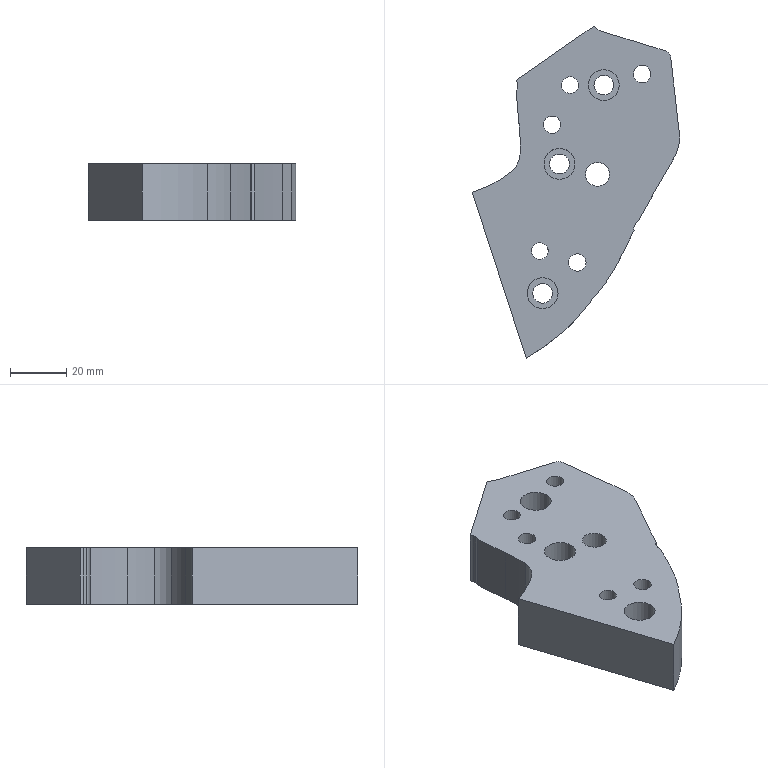Part | NX | features 23 2 | 1 solid | 44 faces | box 73.744 x 117.968 x 20 mm | volume 93989 mm3 | cylinder 30 | plane 14 | commonest cylinder face diameters 4.4 x4 6.2 x3 7 x3 11 x3 6.001 x2 5.6 x1
STEP:
#1=CARTESIAN_POINT('',(1173.772,235.011,-3.5));
#2=VERTEX_POINT('',#1);
#3=CARTESIAN_POINT('',(1169.522,235.011,-3.5));
#4=DIRECTION('',(0.,0.,-1.));
#5=DIRECTION('',(1.,0.,0.));
#6=AXIS2_PLACEMENT_3D('',#3,#4,#5);
#7=CIRCLE('',#6,4.25);
#8=EDGE_CURVE('',#2,#2,#7,.T.);
#9=ORIENTED_EDGE('',*,*,#8,.T.);
#10=EDGE_LOOP('',(#9));
#11=FACE_BOUND('',#10,.T.);
#12=CARTESIAN_POINT('',(1171.238,285.744,-3.5));
#13=VERTEX_POINT('',#12);
#14=CARTESIAN_POINT('',(1168.283,287.713,-3.5));
#15=VERTEX_POINT('',#14);
#16=CARTESIAN_POINT('',(1173.055,291.672,-3.5));
#17=DIRECTION('',(0.,0.,-1.));
#18=DIRECTION('',(-1.,0.,0.));
#19=AXIS2_PLACEMENT_3D('',#16,#17,#18);
#20=CIRCLE('',#19,6.2);
#21=EDGE_CURVE('',#13,#15,#20,.T.);
#22=ORIENTED_EDGE('',*,*,#21,.T.);
#23=CARTESIAN_POINT('',(1140.697,268.486,-3.5));
#24=VERTEX_POINT('',#23);
#25=CARTESIAN_POINT('',(1509.729,525.69,-3.5));
#26=DIRECTION('',(0.8204,0.5718,0.));
#27=VECTOR('',#26,1000.);
#28=LINE('',#25,#27);
#29=EDGE_CURVE('',#24,#15,#28,.T.);
#30=ORIENTED_EDGE('',*,*,#29,.F.);
#31=CARTESIAN_POINT('',(1141.067,267.339,-3.5));
#32=VERTEX_POINT('',#31);
#33=CARTESIAN_POINT('',(1138.868,267.263,-3.5));
#34=DIRECTION('',(0.,0.,-1.));
#35=DIRECTION('',(-1.,0.,0.));
#36=AXIS2_PLACEMENT_3D('',#33,#34,#35);
#37=CIRCLE('',#36,2.2);
#38=EDGE_CURVE('',#24,#32,#37,.T.);
#39=ORIENTED_EDGE('',*,*,#38,.T.);
#40=CARTESIAN_POINT('',(1141.104,266.344,-3.5));
#41=VERTEX_POINT('',#40);
#42=CARTESIAN_POINT('',(1326.856,273.811,-3.5));
#43=DIRECTION('',(0.,0.,1.));
#44=DIRECTION('',(-1.,0.,0.));
#45=AXIS2_PLACEMENT_3D('',#42,#43,#44);
#46=CIRCLE('',#45,185.901);
#47=EDGE_CURVE('',#32,#41,#46,.T.);
#48=ORIENTED_EDGE('',*,*,#47,.T.);
#49=CARTESIAN_POINT('',(1140.666,264.943,-3.5));
#50=VERTEX_POINT('',#49);
#51=CARTESIAN_POINT('',(1138.906,266.263,-3.5));
#52=DIRECTION('',(0.,0.,-1.));
#53=DIRECTION('',(-1.,0.,0.));
#54=AXIS2_PLACEMENT_3D('',#51,#52,#53);
#55=CIRCLE('',#54,2.2);
#56=EDGE_CURVE('',#41,#50,#55,.T.);
#57=ORIENTED_EDGE('',*,*,#56,.T.);
#58=CARTESIAN_POINT('',(1141.757,251.812,-3.5));
#59=VERTEX_POINT('',#58);
#60=CARTESIAN_POINT('',(1326.856,273.811,-3.5));
#61=DIRECTION('',(0.,0.,1.));
#62=DIRECTION('',(-1.,0.,0.));
#63=AXIS2_PLACEMENT_3D('',#60,#61,#62);
#64=CIRCLE('',#63,186.401);
#65=EDGE_CURVE('',#50,#59,#64,.T.);
#66=ORIENTED_EDGE('',*,*,#65,.T.);
#67=CARTESIAN_POINT('',(1141.998,242.228,-3.5));
#68=VERTEX_POINT('',#67);
#69=CARTESIAN_POINT('',(1057.602,244.9,-3.5));
#70=DIRECTION('',(0.,0.,-1.));
#71=DIRECTION('',(-1.,0.,0.));
#72=AXIS2_PLACEMENT_3D('',#69,#70,#71);
#73=CIRCLE('',#72,84.438);
#74=EDGE_CURVE('',#59,#68,#73,.T.);
#75=ORIENTED_EDGE('',*,*,#74,.T.);
#76=CARTESIAN_POINT('',(1139.107,236.023,-3.5));
#77=VERTEX_POINT('',#76);
#78=CARTESIAN_POINT('',(1132.519,242.868,-3.5));
#79=DIRECTION('',(0.,0.,-1.));
#80=DIRECTION('',(-1.,0.,0.));
#81=AXIS2_PLACEMENT_3D('',#78,#79,#80);
#82=CIRCLE('',#81,9.5);
#83=EDGE_CURVE('',#68,#77,#82,.T.);
#84=ORIENTED_EDGE('',*,*,#83,.T.);
#85=CARTESIAN_POINT('',(1131.001,231.048,-3.5));
#86=VERTEX_POINT('',#85);
#87=CARTESIAN_POINT('',(1115.023,266.175,-3.5));
#88=DIRECTION('',(0.,0.,-1.));
#89=DIRECTION('',(-1.,0.,0.));
#90=AXIS2_PLACEMENT_3D('',#87,#88,#89);
#91=CIRCLE('',#90,38.59);
#92=EDGE_CURVE('',#77,#86,#91,.T.);
#93=ORIENTED_EDGE('',*,*,#92,.T.);
#94=CARTESIAN_POINT('',(1126.024,229.046,-3.5));
#95=VERTEX_POINT('',#94);
#96=CARTESIAN_POINT('',(1126.024,229.046,-3.5));
#97=DIRECTION('',(-0.9278,-0.3732,0.));
#98=VECTOR('',#97,1000.);
#99=LINE('',#96,#98);
#100=EDGE_CURVE('',#86,#95,#99,.T.);
#101=ORIENTED_EDGE('',*,*,#100,.T.);
#102=CARTESIAN_POINT('',(1124.992,228.691,-3.5));
#103=VERTEX_POINT('',#102);
#104=CARTESIAN_POINT('',(597.176,1761.975,-3.5));
#105=DIRECTION('',(0.,0.,-1.));
#106=DIRECTION('',(-1.,0.,0.));
#107=AXIS2_PLACEMENT_3D('',#104,#105,#106);
#108=CIRCLE('',#107,1621.589);
#109=EDGE_CURVE('',#95,#103,#108,.T.);
#110=ORIENTED_EDGE('',*,*,#109,.T.);
#111=CARTESIAN_POINT('',(1144.11,169.745,-3.5));
#112=VERTEX_POINT('',#111);
#113=CARTESIAN_POINT('',(1110.681,272.818,-3.5));
#114=DIRECTION('',(0.3085,-0.9512,0.));
#115=VECTOR('',#114,1000.);
#116=LINE('',#113,#115);
#117=EDGE_CURVE('',#103,#112,#116,.T.);
#118=ORIENTED_EDGE('',*,*,#117,.T.);
#119=CARTESIAN_POINT('',(1167.22,190.006,-3.5));
#120=VERTEX_POINT('',#119);
#121=CARTESIAN_POINT('',(1111.807,229.9,-3.5));
#122=DIRECTION('',(0.,0.,1.));
#123=DIRECTION('',(-1.,0.,0.));
#124=AXIS2_PLACEMENT_3D('',#121,#122,#123);
#125=CIRCLE('',#124,68.28);
#126=EDGE_CURVE('',#112,#120,#125,.T.);
#127=ORIENTED_EDGE('',*,*,#126,.T.);
#128=CARTESIAN_POINT('',(1175.627,201.589,-3.5));
#129=VERTEX_POINT('',#128);
#130=CARTESIAN_POINT('',(1118.965,233.873,-3.5));
#131=DIRECTION('',(0.,0.,1.));
#132=DIRECTION('',(-1.,0.,0.));
#133=AXIS2_PLACEMENT_3D('',#130,#131,#132);
#134=CIRCLE('',#133,65.213);
#135=EDGE_CURVE('',#120,#129,#134,.T.);
#136=ORIENTED_EDGE('',*,*,#135,.T.);
#137=CARTESIAN_POINT('',(1182.483,215.038,-3.5));
#138=VERTEX_POINT('',#137);
#139=CARTESIAN_POINT('',(973.133,313.29,-3.5));
#140=DIRECTION('',(0.,0.,1.));
#141=DIRECTION('',(-1.,0.,0.));
#142=AXIS2_PLACEMENT_3D('',#139,#140,#141);
#143=CIRCLE('',#142,231.259);
#144=EDGE_CURVE('',#129,#138,#143,.T.);
#145=ORIENTED_EDGE('',*,*,#144,.T.);
#146=CARTESIAN_POINT('',(1182.612,216.501,-3.5));
#147=VERTEX_POINT('',#146);
#148=CARTESIAN_POINT('',(1184.614,215.586,-3.5));
#149=DIRECTION('',(0.,0.,-1.));
#150=DIRECTION('',(-1.,0.,0.));
#151=AXIS2_PLACEMENT_3D('',#148,#149,#150);
#152=CIRCLE('',#151,2.2);
#153=EDGE_CURVE('',#138,#147,#152,.T.);
#154=ORIENTED_EDGE('',*,*,#153,.T.);
#155=CARTESIAN_POINT('',(1183.03,217.409,-3.5));
#156=VERTEX_POINT('',#155);
#157=CARTESIAN_POINT('',(973.133,313.29,-3.5));
#158=DIRECTION('',(0.,0.,1.));
#159=DIRECTION('',(-1.,0.,0.));
#160=AXIS2_PLACEMENT_3D('',#157,#158,#159);
#161=CIRCLE('',#160,230.759);
#162=EDGE_CURVE('',#147,#156,#161,.T.);
#163=ORIENTED_EDGE('',*,*,#162,.T.);
#164=CARTESIAN_POINT('',(1184.097,218.487,-3.5));
#165=VERTEX_POINT('',#164);
#166=CARTESIAN_POINT('',(1185.031,216.495,-3.5));
#167=DIRECTION('',(0.,0.,-1.));
#168=DIRECTION('',(-1.,0.,0.));
#169=AXIS2_PLACEMENT_3D('',#166,#167,#168);
#170=CIRCLE('',#169,2.2);
#171=EDGE_CURVE('',#156,#165,#170,.T.);
#172=ORIENTED_EDGE('',*,*,#171,.T.);
#173=CARTESIAN_POINT('',(1193.968,236.067,-3.5));
#174=VERTEX_POINT('',#173);
#175=CARTESIAN_POINT('',(1664.113,-39.483,-3.5));
#176=DIRECTION('',(0.,0.,-1.));
#177=DIRECTION('',(-1.,0.,0.));
#178=AXIS2_PLACEMENT_3D('',#175,#176,#177);
#179=CIRCLE('',#178,544.944);
#180=EDGE_CURVE('',#165,#174,#179,.T.);
#181=ORIENTED_EDGE('',*,*,#180,.T.);
#182=CARTESIAN_POINT('',(1197.319,241.921,-3.5));
#183=VERTEX_POINT('',#182);
#184=CARTESIAN_POINT('',(1370.696,544.77,-3.5));
#185=DIRECTION('',(0.4968,0.8678,0.));
#186=VECTOR('',#185,1000.);
#187=LINE('',#184,#186);
#188=EDGE_CURVE('',#174,#183,#187,.T.);
#189=ORIENTED_EDGE('',*,*,#188,.T.);
#190=CARTESIAN_POINT('',(1198.437,250.945,-3.5));
#191=VERTEX_POINT('',#190);
#192=CARTESIAN_POINT('',(1184.704,248.065,-3.5));
#193=DIRECTION('',(0.,0.,1.));
#194=DIRECTION('',(-1.,0.,0.));
#195=AXIS2_PLACEMENT_3D('',#192,#193,#194);
#196=CIRCLE('',#195,14.032);
#197=EDGE_CURVE('',#183,#191,#196,.T.);
#198=ORIENTED_EDGE('',*,*,#197,.T.);
#199=CARTESIAN_POINT('',(1197.911,255.585,-3.5));
#200=VERTEX_POINT('',#199);
#201=CARTESIAN_POINT('',(1183.796,380.097,-3.5));
#202=DIRECTION('',(-0.1126,0.9936,0.));
#203=VECTOR('',#202,1000.);
#204=LINE('',#201,#203);
#205=EDGE_CURVE('',#191,#200,#204,.T.);
#206=ORIENTED_EDGE('',*,*,#205,.T.);
#207=CARTESIAN_POINT('',(1196.117,271.413,-3.5));
#208=VERTEX_POINT('',#207);
#209=CARTESIAN_POINT('',(1183.797,380.099,-3.5));
#210=DIRECTION('',(-0.1126,0.9936,0.));
#211=VECTOR('',#210,1000.);
#212=LINE('',#209,#211);
#213=EDGE_CURVE('',#200,#208,#212,.T.);
#214=ORIENTED_EDGE('',*,*,#213,.T.);
#215=CARTESIAN_POINT('',(1195.536,276.538,-3.5));
#216=VERTEX_POINT('',#215);
#217=CARTESIAN_POINT('',(1183.796,380.094,-3.5));
#218=DIRECTION('',(-0.1126,0.9936,0.));
#219=VECTOR('',#218,1000.);
#220=LINE('',#217,#219);
#221=EDGE_CURVE('',#208,#216,#220,.T.);
#222=ORIENTED_EDGE('',*,*,#221,.T.);
#223=CARTESIAN_POINT('',(1193.574,278.9,-3.5));
#224=VERTEX_POINT('',#223);
#225=CARTESIAN_POINT('',(1192.754,276.223,-3.5));
#226=DIRECTION('',(0.,0.,1.));
#227=DIRECTION('',(-1.,0.,0.));
#228=AXIS2_PLACEMENT_3D('',#225,#226,#227);
#229=CIRCLE('',#228,2.8);
#230=EDGE_CURVE('',#216,#224,#229,.T.);
#231=ORIENTED_EDGE('',*,*,#230,.T.);
#232=CARTESIAN_POINT('',(1182.916,282.165,-3.5));
#233=VERTEX_POINT('',#232);
#234=CARTESIAN_POINT('',(1505.832,183.228,-3.5));
#235=DIRECTION('',(-0.9561,0.2929,0.));
#236=VECTOR('',#235,1000.);
#237=LINE('',#234,#236);
#238=EDGE_CURVE('',#224,#233,#237,.T.);
#239=ORIENTED_EDGE('',*,*,#238,.T.);
#240=CARTESIAN_POINT('',(1505.815,183.216,-3.5));
#241=DIRECTION('',(-0.9561,0.293,0.));
#242=VECTOR('',#241,1000.);
#243=LINE('',#240,#242);
#244=EDGE_CURVE('',#233,#13,#243,.T.);
#245=ORIENTED_EDGE('',*,*,#244,.T.);
#246=EDGE_LOOP('',(#22,#30,#39,#48,#57,#66,#75,#84,#93,#101,#110,#118,#127,#136,#145,#154,#163,#172,#181,#189,#198,#206,#214,#222,#231,#239,#245));
#247=FACE_BOUND('',#246,.T.);
#248=CARTESIAN_POINT('',(1150.492,238.713,-3.5));
#249=VERTEX_POINT('',#248);
#250=CARTESIAN_POINT('',(1155.992,238.713,-3.5));
#251=DIRECTION('',(0.,0.,1.));
#252=DIRECTION('',(-1.,0.,0.));
#253=AXIS2_PLACEMENT_3D('',#250,#251,#252);
#254=CIRCLE('',#253,5.5);
#255=EDGE_CURVE('',#249,#249,#254,.T.);
#256=ORIENTED_EDGE('',*,*,#255,.F.);
#257=EDGE_LOOP('',(#256));
#258=FACE_BOUND('',#257,.T.);
#259=CARTESIAN_POINT('',(1144.492,192.745,-3.5));
#260=VERTEX_POINT('',#259);
#261=CARTESIAN_POINT('',(1149.992,192.745,-3.5));
#262=DIRECTION('',(0.,0.,1.));
#263=DIRECTION('',(-1.,0.,0.));
#264=AXIS2_PLACEMENT_3D('',#261,#262,#263);
#265=CIRCLE('',#264,5.5);
#266=EDGE_CURVE('',#260,#260,#265,.T.);
#267=ORIENTED_EDGE('',*,*,#266,.F.);
#268=EDGE_LOOP('',(#267));
#269=FACE_BOUND('',#268,.T.);
#270=CARTESIAN_POINT('',(1145.992,207.745,-3.5));
#271=VERTEX_POINT('',#270);
#272=CARTESIAN_POINT('',(1148.992,207.745,-3.5));
#273=DIRECTION('',(0.,0.,1.));
#274=DIRECTION('',(-1.,0.,0.));
#275=AXIS2_PLACEMENT_3D('',#272,#273,#274);
#276=CIRCLE('',#275,3.001);
#277=EDGE_CURVE('',#271,#271,#276,.T.);
#278=ORIENTED_EDGE('',*,*,#277,.F.);
#279=EDGE_LOOP('',(#278));
#280=FACE_BOUND('',#279,.T.);
#281=CARTESIAN_POINT('',(1166.236,266.713,-3.5));
#282=VERTEX_POINT('',#281);
#283=CARTESIAN_POINT('',(1171.736,266.713,-3.5));
#284=DIRECTION('',(0.,0.,1.));
#285=DIRECTION('',(-1.,0.,0.));
#286=AXIS2_PLACEMENT_3D('',#283,#284,#285);
#287=CIRCLE('',#286,5.5);
#288=EDGE_CURVE('',#282,#282,#287,.T.);
#289=ORIENTED_EDGE('',*,*,#288,.F.);
#290=EDGE_LOOP('',(#289));
#291=FACE_BOUND('',#290,.T.);
#292=CARTESIAN_POINT('',(1156.735,266.713,-3.5));
#293=VERTEX_POINT('',#292);
#294=CARTESIAN_POINT('',(1159.736,266.713,-3.5));
#295=DIRECTION('',(0.,0.,1.));
#296=DIRECTION('',(-1.,0.,0.));
#297=AXIS2_PLACEMENT_3D('',#294,#295,#296);
#298=CIRCLE('',#297,3.001);
#299=EDGE_CURVE('',#293,#293,#298,.T.);
#300=ORIENTED_EDGE('',*,*,#299,.F.);
#301=EDGE_LOOP('',(#300));
#302=FACE_BOUND('',#301,.T.);
#303=CARTESIAN_POINT('',(1159.26,203.637,-3.5));
#304=VERTEX_POINT('',#303);
#305=CARTESIAN_POINT('',(1162.36,203.637,-3.5));
#306=DIRECTION('',(0.,0.,1.));
#307=DIRECTION('',(-1.,0.,0.));
#308=AXIS2_PLACEMENT_3D('',#305,#306,#307);
#309=CIRCLE('',#308,3.1);
#310=EDGE_CURVE('',#304,#304,#309,.T.);
#311=ORIENTED_EDGE('',*,*,#310,.F.);
#312=EDGE_LOOP('',(#311));
#313=FACE_BOUND('',#312,.T.);
#314=CARTESIAN_POINT('',(1150.26,252.637,-3.5));
#315=VERTEX_POINT('',#314);
#316=CARTESIAN_POINT('',(1153.36,252.637,-3.5));
#317=DIRECTION('',(0.,0.,1.));
#318=DIRECTION('',(-1.,0.,0.));
#319=AXIS2_PLACEMENT_3D('',#316,#317,#318);
#320=CIRCLE('',#319,3.1);
#321=EDGE_CURVE('',#315,#315,#320,.T.);
#322=ORIENTED_EDGE('',*,*,#321,.F.);
#323=EDGE_LOOP('',(#322));
#324=FACE_BOUND('',#323,.T.);
#325=CARTESIAN_POINT('',(1182.26,270.637,-3.5));
#326=VERTEX_POINT('',#325);
#327=CARTESIAN_POINT('',(1185.36,270.637,-3.5));
#328=DIRECTION('',(0.,0.,1.));
#329=DIRECTION('',(-1.,0.,0.));
#330=AXIS2_PLACEMENT_3D('',#327,#328,#329);
#331=CIRCLE('',#330,3.1);
#332=EDGE_CURVE('',#326,#326,#331,.T.);
#333=ORIENTED_EDGE('',*,*,#332,.F.);
#334=EDGE_LOOP('',(#333));
#335=FACE_BOUND('',#334,.T.);
#336=CARTESIAN_POINT('',(1579.908,425.,-3.5));
#337=DIRECTION('',(0.,0.,-1.));
#338=DIRECTION('',(1.,0.,0.));
#339=AXIS2_PLACEMENT_3D('',#336,#337,#338);
#340=PLANE('',#339);
#341=ADVANCED_FACE('',(#11,#247,#258,#269,#280,#291,#302,#313,#324,#335),#340,.F.);
#342=CARTESIAN_POINT('',(1168.283,287.713,-23.5));
#343=VERTEX_POINT('',#342);
#344=CARTESIAN_POINT('',(1140.697,268.486,-23.5));
#345=VERTEX_POINT('',#344);
#346=CARTESIAN_POINT('',(996.344,167.876,-23.5));
#347=DIRECTION('',(-0.8204,-0.5718,0.));
#348=VECTOR('',#347,1000.);
#349=LINE('',#346,#348);
#350=EDGE_CURVE('',#343,#345,#349,.T.);
#351=ORIENTED_EDGE('',*,*,#350,.F.);
#352=CARTESIAN_POINT('',(1171.238,285.744,-23.5));
#353=VERTEX_POINT('',#352);
#354=CARTESIAN_POINT('',(1173.055,291.672,-23.5));
#355=DIRECTION('',(0.,0.,-1.));
#356=DIRECTION('',(-1.,0.,0.));
#357=AXIS2_PLACEMENT_3D('',#354,#355,#356);
#358=CIRCLE('',#357,6.2);
#359=EDGE_CURVE('',#353,#343,#358,.T.);
#360=ORIENTED_EDGE('',*,*,#359,.F.);
#361=CARTESIAN_POINT('',(1182.916,282.165,-23.5));
#362=VERTEX_POINT('',#361);
#363=CARTESIAN_POINT('',(1127.048,299.286,-23.5));
#364=DIRECTION('',(-0.9561,0.293,0.));
#365=VECTOR('',#364,1000.);
#366=LINE('',#363,#365);
#367=EDGE_CURVE('',#362,#353,#366,.T.);
#368=ORIENTED_EDGE('',*,*,#367,.F.);
#369=CARTESIAN_POINT('',(1193.574,278.9,-23.5));
#370=VERTEX_POINT('',#369);
#371=CARTESIAN_POINT('',(1127.048,299.282,-23.5));
#372=DIRECTION('',(0.9561,-0.2929,0.));
#373=VECTOR('',#372,1000.);
#374=LINE('',#371,#373);
#375=EDGE_CURVE('',#362,#370,#374,.T.);
#376=ORIENTED_EDGE('',*,*,#375,.T.);
#377=CARTESIAN_POINT('',(1195.536,276.538,-23.5));
#378=VERTEX_POINT('',#377);
#379=CARTESIAN_POINT('',(1192.754,276.223,-23.5));
#380=DIRECTION('',(0.,0.,1.));
#381=DIRECTION('',(-1.,0.,0.));
#382=AXIS2_PLACEMENT_3D('',#379,#380,#381);
#383=CIRCLE('',#382,2.8);
#384=EDGE_CURVE('',#378,#370,#383,.T.);
#385=ORIENTED_EDGE('',*,*,#384,.F.);
#386=CARTESIAN_POINT('',(1196.117,271.413,-23.5));
#387=VERTEX_POINT('',#386);
#388=CARTESIAN_POINT('',(1188.964,334.504,-23.5));
#389=DIRECTION('',(0.1126,-0.9936,0.));
#390=VECTOR('',#389,1000.);
#391=LINE('',#388,#390);
#392=EDGE_CURVE('',#378,#387,#391,.T.);
#393=ORIENTED_EDGE('',*,*,#392,.T.);
#394=CARTESIAN_POINT('',(1197.911,255.585,-23.5));
#395=VERTEX_POINT('',#394);
#396=CARTESIAN_POINT('',(1188.965,334.504,-23.5));
#397=DIRECTION('',(0.1126,-0.9936,0.));
#398=VECTOR('',#397,1000.);
#399=LINE('',#396,#398);
#400=EDGE_CURVE('',#387,#395,#399,.T.);
#401=ORIENTED_EDGE('',*,*,#400,.T.);
#402=CARTESIAN_POINT('',(1198.437,250.945,-23.5));
#403=VERTEX_POINT('',#402);
#404=CARTESIAN_POINT('',(1188.965,334.504,-23.5));
#405=DIRECTION('',(-0.1126,0.9936,0.));
#406=VECTOR('',#405,1000.);
#407=LINE('',#404,#406);
#408=EDGE_CURVE('',#403,#395,#407,.T.);
#409=ORIENTED_EDGE('',*,*,#408,.F.);
#410=CARTESIAN_POINT('',(1197.319,241.921,-23.5));
#411=VERTEX_POINT('',#410);
#412=CARTESIAN_POINT('',(1184.704,248.065,-23.5));
#413=DIRECTION('',(0.,0.,-1.));
#414=DIRECTION('',(-1.,0.,0.));
#415=AXIS2_PLACEMENT_3D('',#412,#413,#414);
#416=CIRCLE('',#415,14.032);
#417=EDGE_CURVE('',#403,#411,#416,.T.);
#418=ORIENTED_EDGE('',*,*,#417,.T.);
#419=CARTESIAN_POINT('',(1193.968,236.067,-23.5));
#420=VERTEX_POINT('',#419);
#421=CARTESIAN_POINT('',(1219.514,280.69,-23.5));
#422=DIRECTION('',(0.4968,0.8678,0.));
#423=VECTOR('',#422,1000.);
#424=LINE('',#421,#423);
#425=EDGE_CURVE('',#420,#411,#424,.T.);
#426=ORIENTED_EDGE('',*,*,#425,.F.);
#427=CARTESIAN_POINT('',(1184.097,218.487,-23.5));
#428=VERTEX_POINT('',#427);
#429=CARTESIAN_POINT('',(1664.113,-39.483,-23.5));
#430=DIRECTION('',(0.,0.,1.));
#431=DIRECTION('',(-1.,0.,0.));
#432=AXIS2_PLACEMENT_3D('',#429,#430,#431);
#433=CIRCLE('',#432,544.944);
#434=EDGE_CURVE('',#420,#428,#433,.T.);
#435=ORIENTED_EDGE('',*,*,#434,.T.);
#436=CARTESIAN_POINT('',(1183.03,217.409,-23.5));
#437=VERTEX_POINT('',#436);
#438=CARTESIAN_POINT('',(1185.031,216.495,-23.5));
#439=DIRECTION('',(0.,0.,-1.));
#440=DIRECTION('',(-1.,0.,0.));
#441=AXIS2_PLACEMENT_3D('',#438,#439,#440);
#442=CIRCLE('',#441,2.2);
#443=EDGE_CURVE('',#437,#428,#442,.T.);
#444=ORIENTED_EDGE('',*,*,#443,.F.);
#445=CARTESIAN_POINT('',(1182.612,216.501,-23.5));
#446=VERTEX_POINT('',#445);
#447=CARTESIAN_POINT('',(973.133,313.29,-23.5));
#448=DIRECTION('',(0.,0.,-1.));
#449=DIRECTION('',(-1.,0.,0.));
#450=AXIS2_PLACEMENT_3D('',#447,#448,#449);
#451=CIRCLE('',#450,230.759);
#452=EDGE_CURVE('',#437,#446,#451,.T.);
#453=ORIENTED_EDGE('',*,*,#452,.T.);
#454=CARTESIAN_POINT('',(1182.483,215.038,-23.5));
#455=VERTEX_POINT('',#454);
#456=CARTESIAN_POINT('',(1184.614,215.586,-23.5));
#457=DIRECTION('',(0.,0.,-1.));
#458=DIRECTION('',(-1.,0.,0.));
#459=AXIS2_PLACEMENT_3D('',#456,#457,#458);
#460=CIRCLE('',#459,2.2);
#461=EDGE_CURVE('',#455,#446,#460,.T.);
#462=ORIENTED_EDGE('',*,*,#461,.F.);
#463=CARTESIAN_POINT('',(1175.627,201.589,-23.5));
#464=VERTEX_POINT('',#463);
#465=CARTESIAN_POINT('',(973.133,313.29,-23.5));
#466=DIRECTION('',(0.,0.,1.));
#467=DIRECTION('',(-1.,0.,0.));
#468=AXIS2_PLACEMENT_3D('',#465,#466,#467);
#469=CIRCLE('',#468,231.259);
#470=EDGE_CURVE('',#464,#455,#469,.T.);
#471=ORIENTED_EDGE('',*,*,#470,.F.);
#472=CARTESIAN_POINT('',(1167.22,190.006,-23.5));
#473=VERTEX_POINT('',#472);
#474=CARTESIAN_POINT('',(1118.965,233.873,-23.5));
#475=DIRECTION('',(0.,0.,1.));
#476=DIRECTION('',(-1.,0.,0.));
#477=AXIS2_PLACEMENT_3D('',#474,#475,#476);
#478=CIRCLE('',#477,65.213);
#479=EDGE_CURVE('',#473,#464,#478,.T.);
#480=ORIENTED_EDGE('',*,*,#479,.F.);
#481=CARTESIAN_POINT('',(1144.11,169.745,-23.5));
#482=VERTEX_POINT('',#481);
#483=CARTESIAN_POINT('',(1111.807,229.9,-23.5));
#484=DIRECTION('',(0.,0.,-1.));
#485=DIRECTION('',(-1.,0.,0.));
#486=AXIS2_PLACEMENT_3D('',#483,#484,#485);
#487=CIRCLE('',#486,68.28);
#488=EDGE_CURVE('',#473,#482,#487,.T.);
#489=ORIENTED_EDGE('',*,*,#488,.T.);
#490=CARTESIAN_POINT('',(1124.992,228.691,-23.5));
#491=VERTEX_POINT('',#490);
#492=CARTESIAN_POINT('',(1143.323,172.172,-23.5));
#493=DIRECTION('',(-0.3085,0.9512,0.));
#494=VECTOR('',#493,1000.);
#495=LINE('',#492,#494);
#496=EDGE_CURVE('',#482,#491,#495,.T.);
#497=ORIENTED_EDGE('',*,*,#496,.T.);
#498=CARTESIAN_POINT('',(1126.024,229.046,-23.5));
#499=VERTEX_POINT('',#498);
#500=CARTESIAN_POINT('',(597.176,1761.975,-23.5));
#501=DIRECTION('',(0.,0.,-1.));
#502=DIRECTION('',(-1.,0.,0.));
#503=AXIS2_PLACEMENT_3D('',#500,#501,#502);
#504=CIRCLE('',#503,1621.589);
#505=EDGE_CURVE('',#499,#491,#504,.T.);
#506=ORIENTED_EDGE('',*,*,#505,.F.);
#507=CARTESIAN_POINT('',(1131.001,231.048,-23.5));
#508=VERTEX_POINT('',#507);
#509=CARTESIAN_POINT('',(1169.044,246.35,-23.5));
#510=DIRECTION('',(-0.9278,-0.3732,0.));
#511=VECTOR('',#510,1000.);
#512=LINE('',#509,#511);
#513=EDGE_CURVE('',#508,#499,#512,.T.);
#514=ORIENTED_EDGE('',*,*,#513,.F.);
#515=CARTESIAN_POINT('',(1139.107,236.023,-23.5));
#516=VERTEX_POINT('',#515);
#517=CARTESIAN_POINT('',(1115.023,266.175,-23.5));
#518=DIRECTION('',(0.,0.,1.));
#519=DIRECTION('',(-1.,0.,0.));
#520=AXIS2_PLACEMENT_3D('',#517,#518,#519);
#521=CIRCLE('',#520,38.59);
#522=EDGE_CURVE('',#508,#516,#521,.T.);
#523=ORIENTED_EDGE('',*,*,#522,.T.);
#524=CARTESIAN_POINT('',(1141.998,242.228,-23.5));
#525=VERTEX_POINT('',#524);
#526=CARTESIAN_POINT('',(1132.519,242.868,-23.5));
#527=DIRECTION('',(0.,0.,-1.));
#528=DIRECTION('',(-1.,0.,0.));
#529=AXIS2_PLACEMENT_3D('',#526,#527,#528);
#530=CIRCLE('',#529,9.5);
#531=EDGE_CURVE('',#525,#516,#530,.T.);
#532=ORIENTED_EDGE('',*,*,#531,.F.);
#533=CARTESIAN_POINT('',(1141.757,251.812,-23.5));
#534=VERTEX_POINT('',#533);
#535=CARTESIAN_POINT('',(1057.602,244.9,-23.5));
#536=DIRECTION('',(0.,0.,1.));
#537=DIRECTION('',(-1.,0.,0.));
#538=AXIS2_PLACEMENT_3D('',#535,#536,#537);
#539=CIRCLE('',#538,84.438);
#540=EDGE_CURVE('',#525,#534,#539,.T.);
#541=ORIENTED_EDGE('',*,*,#540,.T.);
#542=CARTESIAN_POINT('',(1140.666,264.943,-23.5));
#543=VERTEX_POINT('',#542);
#544=CARTESIAN_POINT('',(1326.856,273.811,-23.5));
#545=DIRECTION('',(0.,0.,-1.));
#546=DIRECTION('',(-1.,0.,0.));
#547=AXIS2_PLACEMENT_3D('',#544,#545,#546);
#548=CIRCLE('',#547,186.401);
#549=EDGE_CURVE('',#534,#543,#548,.T.);
#550=ORIENTED_EDGE('',*,*,#549,.T.);
#551=CARTESIAN_POINT('',(1141.104,266.344,-23.5));
#552=VERTEX_POINT('',#551);
#553=CARTESIAN_POINT('',(1138.906,266.263,-23.5));
#554=DIRECTION('',(0.,0.,-1.));
#555=DIRECTION('',(-1.,0.,0.));
#556=AXIS2_PLACEMENT_3D('',#553,#554,#555);
#557=CIRCLE('',#556,2.2);
#558=EDGE_CURVE('',#552,#543,#557,.T.);
#559=ORIENTED_EDGE('',*,*,#558,.F.);
#560=CARTESIAN_POINT('',(1141.067,267.339,-23.5));
#561=VERTEX_POINT('',#560);
#562=CARTESIAN_POINT('',(1326.856,273.811,-23.5));
#563=DIRECTION('',(0.,0.,-1.));
#564=DIRECTION('',(-1.,0.,0.));
#565=AXIS2_PLACEMENT_3D('',#562,#563,#564);
#566=CIRCLE('',#565,185.901);
#567=EDGE_CURVE('',#552,#561,#566,.T.);
#568=ORIENTED_EDGE('',*,*,#567,.T.);
#569=CARTESIAN_POINT('',(1138.868,267.263,-23.5));
#570=DIRECTION('',(0.,0.,-1.));
#571=DIRECTION('',(-1.,0.,0.));
#572=AXIS2_PLACEMENT_3D('',#569,#570,#571);
#573=CIRCLE('',#572,2.2);
#574=EDGE_CURVE('',#345,#561,#573,.T.);
#575=ORIENTED_EDGE('',*,*,#574,.F.);
#576=EDGE_LOOP('',(#351,#360,#368,#376,#385,#393,#401,#409,#418,#426,#435,#444,#453,#462,#471,#480,#489,#497,#506,#514,#523,#532,#541,#550,#559,#568,#575));
#577=FACE_BOUND('',#576,.T.);
#578=CARTESIAN_POINT('',(1152.492,238.713,-23.5));
#579=VERTEX_POINT('',#578);
#580=CARTESIAN_POINT('',(1155.992,238.713,-23.5));
#581=DIRECTION('',(0.,0.,1.));
#582=DIRECTION('',(-1.,0.,0.));
#583=AXIS2_PLACEMENT_3D('',#580,#581,#582);
#584=CIRCLE('',#583,3.5);
#585=EDGE_CURVE('',#579,#579,#584,.T.);
#586=ORIENTED_EDGE('',*,*,#585,.T.);
#587=EDGE_LOOP('',(#586));
#588=FACE_BOUND('',#587,.T.);
#589=CARTESIAN_POINT('',(1146.492,192.745,-23.5));
#590=VERTEX_POINT('',#589);
#591=CARTESIAN_POINT('',(1149.992,192.745,-23.5));
#592=DIRECTION('',(0.,0.,1.));
#593=DIRECTION('',(-1.,0.,0.));
#594=AXIS2_PLACEMENT_3D('',#591,#592,#593);
#595=CIRCLE('',#594,3.5);
#596=EDGE_CURVE('',#590,#590,#595,.T.);
#597=ORIENTED_EDGE('',*,*,#596,.T.);
#598=EDGE_LOOP('',(#597));
#599=FACE_BOUND('',#598,.T.);
#600=CARTESIAN_POINT('',(1145.992,207.745,-23.5));
#601=VERTEX_POINT('',#600);
#602=CARTESIAN_POINT('',(1148.992,207.745,-23.5));
#603=DIRECTION('',(0.,0.,1.));
#604=DIRECTION('',(-1.,0.,0.));
#605=AXIS2_PLACEMENT_3D('',#602,#603,#604);
#606=CIRCLE('',#605,3.001);
#607=EDGE_CURVE('',#601,#601,#606,.T.);
#608=ORIENTED_EDGE('',*,*,#607,.T.);
#609=EDGE_LOOP('',(#608));
#610=FACE_BOUND('',#609,.T.);
#611=CARTESIAN_POINT('',(1168.236,266.713,-23.5));
#612=VERTEX_POINT('',#611);
#613=CARTESIAN_POINT('',(1171.736,266.713,-23.5));
#614=DIRECTION('',(0.,0.,1.));
#615=DIRECTION('',(-1.,0.,0.));
#616=AXIS2_PLACEMENT_3D('',#613,#614,#615);
#617=CIRCLE('',#616,3.5);
#618=EDGE_CURVE('',#612,#612,#617,.T.);
#619=ORIENTED_EDGE('',*,*,#618,.T.);
#620=EDGE_LOOP('',(#619));
#621=FACE_BOUND('',#620,.T.);
#622=CARTESIAN_POINT('',(1156.735,266.713,-23.5));
#623=VERTEX_POINT('',#622);
#624=CARTESIAN_POINT('',(1159.736,266.713,-23.5));
#625=DIRECTION('',(0.,0.,1.));
#626=DIRECTION('',(-1.,0.,0.));
#627=AXIS2_PLACEMENT_3D('',#624,#625,#626);
#628=CIRCLE('',#627,3.001);
#629=EDGE_CURVE('',#623,#623,#628,.T.);
#630=ORIENTED_EDGE('',*,*,#629,.T.);
#631=EDGE_LOOP('',(#630));
#632=FACE_BOUND('',#631,.T.);
#633=CARTESIAN_POINT('',(1159.26,203.637,-23.5));
#634=VERTEX_POINT('',#633);
#635=CARTESIAN_POINT('',(1162.36,203.637,-23.5));
#636=DIRECTION('',(0.,0.,1.));
#637=DIRECTION('',(-1.,0.,0.));
#638=AXIS2_PLACEMENT_3D('',#635,#636,#637);
#639=CIRCLE('',#638,3.1);
#640=EDGE_CURVE('',#634,#634,#639,.T.);
#641=ORIENTED_EDGE('',*,*,#640,.T.);
#642=EDGE_LOOP('',(#641));
#643=FACE_BOUND('',#642,.T.);
#644=CARTESIAN_POINT('',(1150.26,252.637,-23.5));
#645=VERTEX_POINT('',#644);
#646=CARTESIAN_POINT('',(1153.36,252.637,-23.5));
#647=DIRECTION('',(0.,0.,1.));
#648=DIRECTION('',(-1.,0.,0.));
#649=AXIS2_PLACEMENT_3D('',#646,#647,#648);
#650=CIRCLE('',#649,3.1);
#651=EDGE_CURVE('',#645,#645,#650,.T.);
#652=ORIENTED_EDGE('',*,*,#651,.T.);
#653=EDGE_LOOP('',(#652));
#654=FACE_BOUND('',#653,.T.);
#655=CARTESIAN_POINT('',(1182.26,270.637,-23.5));
#656=VERTEX_POINT('',#655);
#657=CARTESIAN_POINT('',(1185.36,270.637,-23.5));
#658=DIRECTION('',(0.,0.,1.));
#659=DIRECTION('',(-1.,0.,0.));
#660=AXIS2_PLACEMENT_3D('',#657,#658,#659);
#661=CIRCLE('',#660,3.1);
#662=EDGE_CURVE('',#656,#656,#661,.T.);
#663=ORIENTED_EDGE('',*,*,#662,.T.);
#664=EDGE_LOOP('',(#663));
#665=FACE_BOUND('',#664,.T.);
#666=CARTESIAN_POINT('',(1165.272,235.011,-23.5));
#667=VERTEX_POINT('',#666);
#668=CARTESIAN_POINT('',(1169.522,235.011,-23.5));
#669=DIRECTION('',(0.,0.,1.));
#670=DIRECTION('',(-1.,0.,0.));
#671=AXIS2_PLACEMENT_3D('',#668,#669,#670);
#672=CIRCLE('',#671,4.25);
#673=EDGE_CURVE('',#667,#667,#672,.T.);
#674=ORIENTED_EDGE('',*,*,#673,.T.);
#675=EDGE_LOOP('',(#674));
#676=FACE_BOUND('',#675,.T.);
#677=CARTESIAN_POINT('',(1021.,132.5,-23.5));
#678=DIRECTION('',(0.,0.,-1.));
#679=DIRECTION('',(1.,0.,0.));
#680=AXIS2_PLACEMENT_3D('',#677,#678,#679);
#681=PLANE('',#680);
#682=ADVANCED_FACE('',(#577,#588,#599,#610,#621,#632,#643,#654,#665,#676),#681,.T.);
#683=ORIENTED_EDGE('',*,*,#479,.T.);
#684=CARTESIAN_POINT('',(1175.627,201.589,-43.));
#685=DIRECTION('',(0.,0.,-1.));
#686=VECTOR('',#685,1000.);
#687=LINE('',#684,#686);
#688=EDGE_CURVE('',#129,#464,#687,.T.);
#689=ORIENTED_EDGE('',*,*,#688,.F.);
#690=ORIENTED_EDGE('',*,*,#135,.F.);
#691=CARTESIAN_POINT('',(1167.22,190.006,-43.));
#692=DIRECTION('',(0.,0.,-1.));
#693=VECTOR('',#692,1000.);
#694=LINE('',#691,#693);
#695=EDGE_CURVE('',#120,#473,#694,.T.);
#696=ORIENTED_EDGE('',*,*,#695,.T.);
#697=EDGE_LOOP('',(#683,#689,#690,#696));
#698=FACE_BOUND('',#697,.T.);
#699=CARTESIAN_POINT('',(1118.965,233.873,-43.));
#700=DIRECTION('',(0.,0.,1.));
#701=DIRECTION('',(-1.,0.,0.));
#702=AXIS2_PLACEMENT_3D('',#699,#700,#701);
#703=CYLINDRICAL_SURFACE('',#702,65.213);
#704=ADVANCED_FACE('',(#698),#703,.T.);
#705=ORIENTED_EDGE('',*,*,#470,.T.);
#706=CARTESIAN_POINT('',(1182.483,215.038,-43.));
#707=DIRECTION('',(0.,0.,-1.));
#708=VECTOR('',#707,1000.);
#709=LINE('',#706,#708);
#710=EDGE_CURVE('',#138,#455,#709,.T.);
#711=ORIENTED_EDGE('',*,*,#710,.F.);
#712=ORIENTED_EDGE('',*,*,#144,.F.);
#713=ORIENTED_EDGE('',*,*,#688,.T.);
#714=EDGE_LOOP('',(#705,#711,#712,#713));
#715=FACE_BOUND('',#714,.T.);
#716=CARTESIAN_POINT('',(973.133,313.29,-43.));
#717=DIRECTION('',(0.,0.,1.));
#718=DIRECTION('',(-1.,0.,0.));
#719=AXIS2_PLACEMENT_3D('',#716,#717,#718);
#720=CYLINDRICAL_SURFACE('',#719,231.259);
#721=ADVANCED_FACE('',(#715),#720,.T.);
#722=ORIENTED_EDGE('',*,*,#461,.T.);
#723=CARTESIAN_POINT('',(1182.612,216.501,-23.5));
#724=CARTESIAN_POINT('',(1182.612,216.501,-16.833));
#725=CARTESIAN_POINT('',(1182.612,216.501,-10.167));
#726=CARTESIAN_POINT('',(1182.612,216.501,-3.5));
#727=B_SPLINE_CURVE_WITH_KNOTS('',3,(#723,#724,#725,#726),.UNSPECIFIED.,.F.,.F.,(4,4),(0.,1.),.UNSPECIFIED.);
#728=EDGE_CURVE('',#147,#446,#727,.F.);
#729=ORIENTED_EDGE('',*,*,#728,.F.);
#730=ORIENTED_EDGE('',*,*,#153,.F.);
#731=ORIENTED_EDGE('',*,*,#710,.T.);
#732=EDGE_LOOP('',(#722,#729,#730,#731));
#733=FACE_BOUND('',#732,.T.);
#734=CARTESIAN_POINT('',(1184.614,215.586,-43.));
#735=DIRECTION('',(0.,0.,1.));
#736=DIRECTION('',(-1.,0.,0.));
#737=AXIS2_PLACEMENT_3D('',#734,#735,#736);
#738=CYLINDRICAL_SURFACE('',#737,2.2);
#739=ADVANCED_FACE('',(#733),#738,.F.);
#740=ORIENTED_EDGE('',*,*,#452,.F.);
#741=CARTESIAN_POINT('',(1183.03,217.409,-43.));
#742=DIRECTION('',(0.,0.,-1.));
#743=VECTOR('',#742,1000.);
#744=LINE('',#741,#743);
#745=EDGE_CURVE('',#156,#437,#744,.T.);
#746=ORIENTED_EDGE('',*,*,#745,.F.);
#747=ORIENTED_EDGE('',*,*,#162,.F.);
#748=ORIENTED_EDGE('',*,*,#728,.T.);
#749=EDGE_LOOP('',(#740,#746,#747,#748));
#750=FACE_BOUND('',#749,.T.);
#751=CARTESIAN_POINT('',(973.133,313.29,-43.));
#752=DIRECTION('',(0.,0.,1.));
#753=DIRECTION('',(-1.,0.,0.));
#754=AXIS2_PLACEMENT_3D('',#751,#752,#753);
#755=CYLINDRICAL_SURFACE('',#754,230.759);
#756=ADVANCED_FACE('',(#750),#755,.T.);
#757=ORIENTED_EDGE('',*,*,#443,.T.);
#758=CARTESIAN_POINT('',(1184.097,218.487,-43.));
#759=DIRECTION('',(0.,0.,-1.));
#760=VECTOR('',#759,1000.);
#761=LINE('',#758,#760);
#762=EDGE_CURVE('',#165,#428,#761,.T.);
#763=ORIENTED_EDGE('',*,*,#762,.F.);
#764=ORIENTED_EDGE('',*,*,#171,.F.);
#765=ORIENTED_EDGE('',*,*,#745,.T.);
#766=EDGE_LOOP('',(#757,#763,#764,#765));
#767=FACE_BOUND('',#766,.T.);
#768=CARTESIAN_POINT('',(1185.031,216.495,-43.));
#769=DIRECTION('',(0.,0.,1.));
#770=DIRECTION('',(-1.,0.,0.));
#771=AXIS2_PLACEMENT_3D('',#768,#769,#770);
#772=CYLINDRICAL_SURFACE('',#771,2.2);
#773=ADVANCED_FACE('',(#767),#772,.F.);
#774=ORIENTED_EDGE('',*,*,#434,.F.);
#775=CARTESIAN_POINT('',(1193.968,236.067,-43.));
#776=DIRECTION('',(0.,0.,-1.));
#777=VECTOR('',#776,1000.);
#778=LINE('',#775,#777);
#779=EDGE_CURVE('',#174,#420,#778,.T.);
#780=ORIENTED_EDGE('',*,*,#779,.F.);
#781=ORIENTED_EDGE('',*,*,#180,.F.);
#782=ORIENTED_EDGE('',*,*,#762,.T.);
#783=EDGE_LOOP('',(#774,#780,#781,#782));
#784=FACE_BOUND('',#783,.T.);
#785=CARTESIAN_POINT('',(1664.113,-39.483,-43.));
#786=DIRECTION('',(0.,0.,1.));
#787=DIRECTION('',(-1.,0.,0.));
#788=AXIS2_PLACEMENT_3D('',#785,#786,#787);
#789=CYLINDRICAL_SURFACE('',#788,544.944);
#790=ADVANCED_FACE('',(#784),#789,.F.);
#791=ORIENTED_EDGE('',*,*,#425,.T.);
#792=CARTESIAN_POINT('',(1197.319,241.921,-13.5));
#793=DIRECTION('',(0.,0.,-1.));
#794=VECTOR('',#793,1000.);
#795=LINE('',#792,#794);
#796=EDGE_CURVE('',#183,#411,#795,.T.);
#797=ORIENTED_EDGE('',*,*,#796,.F.);
#798=ORIENTED_EDGE('',*,*,#188,.F.);
#799=ORIENTED_EDGE('',*,*,#779,.T.);
#800=EDGE_LOOP('',(#791,#797,#798,#799));
#801=FACE_BOUND('',#800,.T.);
#802=CARTESIAN_POINT('',(1193.968,236.067,-43.));
#803=DIRECTION('',(0.8678,-0.4968,0.));
#804=DIRECTION('',(-0.4968,-0.8678,0.));
#805=AXIS2_PLACEMENT_3D('',#802,#803,#804);
#806=PLANE('',#805);
#807=ADVANCED_FACE('',(#801),#806,.T.);
#808=ORIENTED_EDGE('',*,*,#417,.F.);
#809=CARTESIAN_POINT('',(1198.437,250.945,-3.5));
#810=DIRECTION('',(0.,0.,1.));
#811=VECTOR('',#810,1000.);
#812=LINE('',#809,#811);
#813=EDGE_CURVE('',#191,#403,#812,.F.);
#814=ORIENTED_EDGE('',*,*,#813,.F.);
#815=ORIENTED_EDGE('',*,*,#197,.F.);
#816=ORIENTED_EDGE('',*,*,#796,.T.);
#817=EDGE_LOOP('',(#808,#814,#815,#816));
#818=FACE_BOUND('',#817,.T.);
#819=CARTESIAN_POINT('',(1184.704,248.065,-43.));
#820=DIRECTION('',(0.,0.,1.));
#821=DIRECTION('',(-1.,0.,0.));
#822=AXIS2_PLACEMENT_3D('',#819,#820,#821);
#823=CYLINDRICAL_SURFACE('',#822,14.032);
#824=ADVANCED_FACE('',(#818),#823,.T.);
#825=ORIENTED_EDGE('',*,*,#408,.T.);
#826=CARTESIAN_POINT('',(1197.911,255.585,-43.));
#827=DIRECTION('',(0.,0.,-1.));
#828=VECTOR('',#827,1000.);
#829=LINE('',#826,#828);
#830=EDGE_CURVE('',#200,#395,#829,.T.);
#831=ORIENTED_EDGE('',*,*,#830,.F.);
#832=ORIENTED_EDGE('',*,*,#205,.F.);
#833=ORIENTED_EDGE('',*,*,#813,.T.);
#834=EDGE_LOOP('',(#825,#831,#832,#833));
#835=FACE_BOUND('',#834,.T.);
#836=CARTESIAN_POINT('',(1198.437,250.946,-43.));
#837=DIRECTION('',(0.9936,0.1126,0.));
#838=DIRECTION('',(0.1126,-0.9936,0.));
#839=AXIS2_PLACEMENT_3D('',#836,#837,#838);
#840=PLANE('',#839);
#841=ADVANCED_FACE('',(#835),#840,.T.);
#842=ORIENTED_EDGE('',*,*,#400,.F.);
#843=CARTESIAN_POINT('',(1196.117,271.413,-43.));
#844=DIRECTION('',(0.,0.,-1.));
#845=VECTOR('',#844,1000.);
#846=LINE('',#843,#845);
#847=EDGE_CURVE('',#208,#387,#846,.T.);
#848=ORIENTED_EDGE('',*,*,#847,.F.);
#849=ORIENTED_EDGE('',*,*,#213,.F.);
#850=ORIENTED_EDGE('',*,*,#830,.T.);
#851=EDGE_LOOP('',(#842,#848,#849,#850));
#852=FACE_BOUND('',#851,.T.);
#853=CARTESIAN_POINT('',(1197.911,255.585,-43.));
#854=DIRECTION('',(0.9936,0.1126,0.));
#855=DIRECTION('',(0.1126,-0.9936,0.));
#856=AXIS2_PLACEMENT_3D('',#853,#854,#855);
#857=PLANE('',#856);
#858=ADVANCED_FACE('',(#852),#857,.T.);
#859=ORIENTED_EDGE('',*,*,#392,.F.);
#860=CARTESIAN_POINT('',(1195.536,276.538,-43.));
#861=DIRECTION('',(0.,0.,-1.));
#862=VECTOR('',#861,1000.);
#863=LINE('',#860,#862);
#864=EDGE_CURVE('',#216,#378,#863,.T.);
#865=ORIENTED_EDGE('',*,*,#864,.F.);
#866=ORIENTED_EDGE('',*,*,#221,.F.);
#867=ORIENTED_EDGE('',*,*,#847,.T.);
#868=EDGE_LOOP('',(#859,#865,#866,#867));
#869=FACE_BOUND('',#868,.T.);
#870=CARTESIAN_POINT('',(1196.117,271.413,-43.));
#871=DIRECTION('',(0.9936,0.1126,0.));
#872=DIRECTION('',(0.1126,-0.9936,0.));
#873=AXIS2_PLACEMENT_3D('',#870,#871,#872);
#874=PLANE('',#873);
#875=ADVANCED_FACE('',(#869),#874,.T.);
#876=ORIENTED_EDGE('',*,*,#384,.T.);
#877=CARTESIAN_POINT('',(1193.574,278.9,-43.));
#878=DIRECTION('',(0.,0.,-1.));
#879=VECTOR('',#878,1000.);
#880=LINE('',#877,#879);
#881=EDGE_CURVE('',#224,#370,#880,.T.);
#882=ORIENTED_EDGE('',*,*,#881,.F.);
#883=ORIENTED_EDGE('',*,*,#230,.F.);
#884=ORIENTED_EDGE('',*,*,#864,.T.);
#885=EDGE_LOOP('',(#876,#882,#883,#884));
#886=FACE_BOUND('',#885,.T.);
#887=CARTESIAN_POINT('',(1192.754,276.223,-43.));
#888=DIRECTION('',(0.,0.,1.));
#889=DIRECTION('',(-1.,0.,0.));
#890=AXIS2_PLACEMENT_3D('',#887,#888,#889);
#891=CYLINDRICAL_SURFACE('',#890,2.8);
#892=ADVANCED_FACE('',(#886),#891,.T.);
#893=ORIENTED_EDGE('',*,*,#375,.F.);
#894=CARTESIAN_POINT('',(1182.916,282.165,-43.));
#895=DIRECTION('',(0.,0.,-1.));
#896=VECTOR('',#895,1000.);
#897=LINE('',#894,#896);
#898=EDGE_CURVE('',#233,#362,#897,.T.);
#899=ORIENTED_EDGE('',*,*,#898,.F.);
#900=ORIENTED_EDGE('',*,*,#238,.F.);
#901=ORIENTED_EDGE('',*,*,#881,.T.);
#902=EDGE_LOOP('',(#893,#899,#900,#901));
#903=FACE_BOUND('',#902,.T.);
#904=CARTESIAN_POINT('',(1193.574,278.9,-43.));
#905=DIRECTION('',(0.2929,0.9561,0.));
#906=DIRECTION('',(0.9561,-0.2929,0.));
#907=AXIS2_PLACEMENT_3D('',#904,#905,#906);
#908=PLANE('',#907);
#909=ADVANCED_FACE('',(#903),#908,.T.);
#910=ORIENTED_EDGE('',*,*,#367,.T.);
#911=CARTESIAN_POINT('',(1171.238,285.744,-43.));
#912=DIRECTION('',(0.,0.,-1.));
#913=VECTOR('',#912,1000.);
#914=LINE('',#911,#913);
#915=EDGE_CURVE('',#13,#353,#914,.T.);
#916=ORIENTED_EDGE('',*,*,#915,.F.);
#917=ORIENTED_EDGE('',*,*,#244,.F.);
#918=ORIENTED_EDGE('',*,*,#898,.T.);
#919=EDGE_LOOP('',(#910,#916,#917,#918));
#920=FACE_BOUND('',#919,.T.);
#921=CARTESIAN_POINT('',(1182.916,282.165,-43.));
#922=DIRECTION('',(0.293,0.9561,0.));
#923=DIRECTION('',(0.9561,-0.293,0.));
#924=AXIS2_PLACEMENT_3D('',#921,#922,#923);
#925=PLANE('',#924);
#926=ADVANCED_FACE('',(#920),#925,.T.);
#927=CARTESIAN_POINT('',(1168.283,287.713,-43.));
#928=DIRECTION('',(0.,0.,-1.));
#929=VECTOR('',#928,1000.);
#930=LINE('',#927,#929);
#931=EDGE_CURVE('',#15,#343,#930,.T.);
#932=ORIENTED_EDGE('',*,*,#931,.F.);
#933=ORIENTED_EDGE('',*,*,#21,.F.);
#934=ORIENTED_EDGE('',*,*,#915,.T.);
#935=ORIENTED_EDGE('',*,*,#359,.T.);
#936=EDGE_LOOP('',(#932,#933,#934,#935));
#937=FACE_BOUND('',#936,.T.);
#938=CARTESIAN_POINT('',(1173.055,291.672,-43.));
#939=DIRECTION('',(0.,0.,1.));
#940=DIRECTION('',(-1.,0.,0.));
#941=AXIS2_PLACEMENT_3D('',#938,#939,#940);
#942=CYLINDRICAL_SURFACE('',#941,6.2);
#943=ADVANCED_FACE('',(#937),#942,.F.);
#944=ORIENTED_EDGE('',*,*,#38,.F.);
#945=CARTESIAN_POINT('',(1140.697,268.486,-43.001));
#946=DIRECTION('',(0.,0.,-1.));
#947=VECTOR('',#946,1000.);
#948=LINE('',#945,#947);
#949=EDGE_CURVE('',#24,#345,#948,.T.);
#950=ORIENTED_EDGE('',*,*,#949,.T.);
#951=ORIENTED_EDGE('',*,*,#574,.T.);
#952=CARTESIAN_POINT('',(1141.067,267.339,-43.001));
#953=DIRECTION('',(0.,0.,1.));
#954=VECTOR('',#953,1000.);
#955=LINE('',#952,#954);
#956=EDGE_CURVE('',#561,#32,#955,.T.);
#957=ORIENTED_EDGE('',*,*,#956,.T.);
#958=EDGE_LOOP('',(#944,#950,#951,#957));
#959=FACE_BOUND('',#958,.T.);
#960=CARTESIAN_POINT('',(1138.868,267.263,-43.001));
#961=DIRECTION('',(0.,0.,1.));
#962=DIRECTION('',(-1.,0.,0.));
#963=AXIS2_PLACEMENT_3D('',#960,#961,#962);
#964=CYLINDRICAL_SURFACE('',#963,2.2);
#965=ADVANCED_FACE('',(#959),#964,.F.);
#966=ORIENTED_EDGE('',*,*,#956,.F.);
#967=ORIENTED_EDGE('',*,*,#567,.F.);
#968=CARTESIAN_POINT('',(1141.104,266.344,-43.001));
#969=DIRECTION('',(0.,0.,1.));
#970=VECTOR('',#969,1000.);
#971=LINE('',#968,#970);
#972=EDGE_CURVE('',#552,#41,#971,.T.);
#973=ORIENTED_EDGE('',*,*,#972,.T.);
#974=ORIENTED_EDGE('',*,*,#47,.F.);
#975=EDGE_LOOP('',(#966,#967,#973,#974));
#976=FACE_BOUND('',#975,.T.);
#977=CARTESIAN_POINT('',(1326.856,273.811,-43.001));
#978=DIRECTION('',(0.,0.,1.));
#979=DIRECTION('',(-1.,0.,0.));
#980=AXIS2_PLACEMENT_3D('',#977,#978,#979);
#981=CYLINDRICAL_SURFACE('',#980,185.901);
#982=ADVANCED_FACE('',(#976),#981,.T.);
#983=ORIENTED_EDGE('',*,*,#972,.F.);
#984=ORIENTED_EDGE('',*,*,#558,.T.);
#985=CARTESIAN_POINT('',(1140.666,264.943,-43.001));
#986=DIRECTION('',(0.,0.,1.));
#987=VECTOR('',#986,1000.);
#988=LINE('',#985,#987);
#989=EDGE_CURVE('',#543,#50,#988,.T.);
#990=ORIENTED_EDGE('',*,*,#989,.T.);
#991=ORIENTED_EDGE('',*,*,#56,.F.);
#992=EDGE_LOOP('',(#983,#984,#990,#991));
#993=FACE_BOUND('',#992,.T.);
#994=CARTESIAN_POINT('',(1138.906,266.263,-43.001));
#995=DIRECTION('',(0.,0.,1.));
#996=DIRECTION('',(-1.,0.,0.));
#997=AXIS2_PLACEMENT_3D('',#994,#995,#996);
#998=CYLINDRICAL_SURFACE('',#997,2.2);
#999=ADVANCED_FACE('',(#993),#998,.F.);
#1000=ORIENTED_EDGE('',*,*,#989,.F.);
#1001=ORIENTED_EDGE('',*,*,#549,.F.);
#1002=CARTESIAN_POINT('',(1141.757,251.812,-43.001));
#1003=DIRECTION('',(0.,0.,1.));
#1004=VECTOR('',#1003,1000.);
#1005=LINE('',#1002,#1004);
#1006=EDGE_CURVE('',#534,#59,#1005,.T.);
#1007=ORIENTED_EDGE('',*,*,#1006,.T.);
#1008=ORIENTED_EDGE('',*,*,#65,.F.);
#1009=EDGE_LOOP('',(#1000,#1001,#1007,#1008));
#1010=FACE_BOUND('',#1009,.T.);
#1011=CARTESIAN_POINT('',(1326.856,273.811,-43.001));
#1012=DIRECTION('',(0.,0.,1.));
#1013=DIRECTION('',(-1.,0.,0.));
#1014=AXIS2_PLACEMENT_3D('',#1011,#1012,#1013);
#1015=CYLINDRICAL_SURFACE('',#1014,186.401);
#1016=ADVANCED_FACE('',(#1010),#1015,.T.);
#1017=ORIENTED_EDGE('',*,*,#1006,.F.);
#1018=ORIENTED_EDGE('',*,*,#540,.F.);
#1019=CARTESIAN_POINT('',(1141.998,242.228,-43.001));
#1020=DIRECTION('',(0.,0.,1.));
#1021=VECTOR('',#1020,1000.);
#1022=LINE('',#1019,#1021);
#1023=EDGE_CURVE('',#525,#68,#1022,.T.);
#1024=ORIENTED_EDGE('',*,*,#1023,.T.);
#1025=ORIENTED_EDGE('',*,*,#74,.F.);
#1026=EDGE_LOOP('',(#1017,#1018,#1024,#1025));
#1027=FACE_BOUND('',#1026,.T.);
#1028=CARTESIAN_POINT('',(1057.602,244.9,-43.001));
#1029=DIRECTION('',(0.,0.,1.));
#1030=DIRECTION('',(-1.,0.,0.));
#1031=AXIS2_PLACEMENT_3D('',#1028,#1029,#1030);
#1032=CYLINDRICAL_SURFACE('',#1031,84.438);
#1033=ADVANCED_FACE('',(#1027),#1032,.F.);
#1034=ORIENTED_EDGE('',*,*,#1023,.F.);
#1035=ORIENTED_EDGE('',*,*,#531,.T.);
#1036=CARTESIAN_POINT('',(1139.107,236.023,-43.001));
#1037=DIRECTION('',(0.,0.,1.));
#1038=VECTOR('',#1037,1000.);
#1039=LINE('',#1036,#1038);
#1040=EDGE_CURVE('',#516,#77,#1039,.T.);
#1041=ORIENTED_EDGE('',*,*,#1040,.T.);
#1042=ORIENTED_EDGE('',*,*,#83,.F.);
#1043=EDGE_LOOP('',(#1034,#1035,#1041,#1042));
#1044=FACE_BOUND('',#1043,.T.);
#1045=CARTESIAN_POINT('',(1132.519,242.868,-43.001));
#1046=DIRECTION('',(0.,0.,1.));
#1047=DIRECTION('',(-1.,0.,0.));
#1048=AXIS2_PLACEMENT_3D('',#1045,#1046,#1047);
#1049=CYLINDRICAL_SURFACE('',#1048,9.5);
#1050=ADVANCED_FACE('',(#1044),#1049,.F.);
#1051=ORIENTED_EDGE('',*,*,#1040,.F.);
#1052=ORIENTED_EDGE('',*,*,#522,.F.);
#1053=CARTESIAN_POINT('',(1131.001,231.048,-43.001));
#1054=DIRECTION('',(0.,0.,1.));
#1055=VECTOR('',#1054,1000.);
#1056=LINE('',#1053,#1055);
#1057=EDGE_CURVE('',#508,#86,#1056,.T.);
#1058=ORIENTED_EDGE('',*,*,#1057,.T.);
#1059=ORIENTED_EDGE('',*,*,#92,.F.);
#1060=EDGE_LOOP('',(#1051,#1052,#1058,#1059));
#1061=FACE_BOUND('',#1060,.T.);
#1062=CARTESIAN_POINT('',(1115.023,266.175,-43.001));
#1063=DIRECTION('',(0.,0.,1.));
#1064=DIRECTION('',(-1.,0.,0.));
#1065=AXIS2_PLACEMENT_3D('',#1062,#1063,#1064);
#1066=CYLINDRICAL_SURFACE('',#1065,38.59);
#1067=ADVANCED_FACE('',(#1061),#1066,.F.);
#1068=ORIENTED_EDGE('',*,*,#1057,.F.);
#1069=ORIENTED_EDGE('',*,*,#513,.T.);
#1070=CARTESIAN_POINT('',(1126.024,229.046,-43.001));
#1071=DIRECTION('',(0.,0.,1.));
#1072=VECTOR('',#1071,1000.);
#1073=LINE('',#1070,#1072);
#1074=EDGE_CURVE('',#499,#95,#1073,.T.);
#1075=ORIENTED_EDGE('',*,*,#1074,.T.);
#1076=ORIENTED_EDGE('',*,*,#100,.F.);
#1077=EDGE_LOOP('',(#1068,#1069,#1075,#1076));
#1078=FACE_BOUND('',#1077,.T.);
#1079=CARTESIAN_POINT('',(1126.024,229.046,-43.001));
#1080=DIRECTION('',(0.3732,-0.9278,0.));
#1081=DIRECTION('',(-0.9278,-0.3732,0.));
#1082=AXIS2_PLACEMENT_3D('',#1079,#1080,#1081);
#1083=PLANE('',#1082);
#1084=ADVANCED_FACE('',(#1078),#1083,.F.);
#1085=CARTESIAN_POINT('',(1144.11,169.745,-43.));
#1086=DIRECTION('',(0.,0.,1.));
#1087=VECTOR('',#1086,1000.);
#1088=LINE('',#1085,#1087);
#1089=EDGE_CURVE('',#482,#112,#1088,.T.);
#1090=ORIENTED_EDGE('',*,*,#1089,.F.);
#1091=ORIENTED_EDGE('',*,*,#488,.F.);
#1092=ORIENTED_EDGE('',*,*,#695,.F.);
#1093=ORIENTED_EDGE('',*,*,#126,.F.);
#1094=EDGE_LOOP('',(#1090,#1091,#1092,#1093));
#1095=FACE_BOUND('',#1094,.T.);
#1096=CARTESIAN_POINT('',(1111.807,229.9,-43.));
#1097=DIRECTION('',(0.,0.,1.));
#1098=DIRECTION('',(-1.,0.,0.));
#1099=AXIS2_PLACEMENT_3D('',#1096,#1097,#1098);
#1100=CYLINDRICAL_SURFACE('',#1099,68.28);
#1101=ADVANCED_FACE('',(#1095),#1100,.T.);
#1102=CARTESIAN_POINT('',(1124.992,228.691,-43.));
#1103=DIRECTION('',(0.,0.,-1.));
#1104=VECTOR('',#1103,1000.);
#1105=LINE('',#1102,#1104);
#1106=EDGE_CURVE('',#103,#491,#1105,.T.);
#1107=ORIENTED_EDGE('',*,*,#1106,.F.);
#1108=ORIENTED_EDGE('',*,*,#109,.F.);
#1109=ORIENTED_EDGE('',*,*,#1074,.F.);
#1110=ORIENTED_EDGE('',*,*,#505,.T.);
#1111=EDGE_LOOP('',(#1107,#1108,#1109,#1110));
#1112=FACE_BOUND('',#1111,.T.);
#1113=CARTESIAN_POINT('',(597.176,1761.975,-43.));
#1114=DIRECTION('',(0.,0.,1.));
#1115=DIRECTION('',(-1.,0.,0.));
#1116=AXIS2_PLACEMENT_3D('',#1113,#1114,#1115);
#1117=CYLINDRICAL_SURFACE('',#1116,1621.589);
#1118=ADVANCED_FACE('',(#1112),#1117,.F.);
#1119=ORIENTED_EDGE('',*,*,#1106,.T.);
#1120=ORIENTED_EDGE('',*,*,#496,.F.);
#1121=ORIENTED_EDGE('',*,*,#1089,.T.);
#1122=ORIENTED_EDGE('',*,*,#117,.F.);
#1123=EDGE_LOOP('',(#1119,#1120,#1121,#1122));
#1124=FACE_BOUND('',#1123,.T.);
#1125=CARTESIAN_POINT('',(1157.,130.,-47.001));
#1126=DIRECTION('',(0.9512,0.3085,0.));
#1127=DIRECTION('',(0.3085,-0.9512,0.));
#1128=AXIS2_PLACEMENT_3D('',#1125,#1126,#1127);
#1129=PLANE('',#1128);
#1130=ADVANCED_FACE('',(#1124),#1129,.F.);
#1131=ORIENTED_EDGE('',*,*,#931,.T.);
#1132=ORIENTED_EDGE('',*,*,#350,.T.);
#1133=ORIENTED_EDGE('',*,*,#949,.F.);
#1134=ORIENTED_EDGE('',*,*,#29,.T.);
#1135=EDGE_LOOP('',(#1131,#1132,#1133,#1134));
#1136=FACE_BOUND('',#1135,.T.);
#1137=CARTESIAN_POINT('',(1140.,268.,-47.001));
#1138=DIRECTION('',(0.5718,-0.8204,0.));
#1139=DIRECTION('',(-0.8204,-0.5718,0.));
#1140=AXIS2_PLACEMENT_3D('',#1137,#1138,#1139);
#1141=PLANE('',#1140);
#1142=ADVANCED_FACE('',(#1136),#1141,.F.);
#1143=CARTESIAN_POINT('',(1161.492,238.713,-12.497));
#1144=VERTEX_POINT('',#1143);
#1145=CARTESIAN_POINT('',(1155.992,238.713,-12.497));
#1146=DIRECTION('',(0.,0.,1.));
#1147=DIRECTION('',(1.,0.,0.));
#1148=AXIS2_PLACEMENT_3D('',#1145,#1146,#1147);
#1149=CIRCLE('',#1148,5.5);
#1150=EDGE_CURVE('',#1144,#1144,#1149,.T.);
#1151=ORIENTED_EDGE('',*,*,#1150,.F.);
#1152=EDGE_LOOP('',(#1151));
#1153=FACE_BOUND('',#1152,.T.);
#1154=ORIENTED_EDGE('',*,*,#255,.T.);
#1155=EDGE_LOOP('',(#1154));
#1156=FACE_BOUND('',#1155,.T.);
#1157=CARTESIAN_POINT('',(1155.992,238.713,-3.497));
#1158=DIRECTION('',(0.,0.,-1.));
#1159=DIRECTION('',(-1.,0.,0.));
#1160=AXIS2_PLACEMENT_3D('',#1157,#1158,#1159);
#1161=CYLINDRICAL_SURFACE('',#1160,5.5);
#1162=ADVANCED_FACE('',(#1153,#1156),#1161,.F.);
#1163=ORIENTED_EDGE('',*,*,#585,.F.);
#1164=EDGE_LOOP('',(#1163));
#1165=FACE_BOUND('',#1164,.T.);
#1166=CARTESIAN_POINT('',(1152.492,238.713,-12.497));
#1167=VERTEX_POINT('',#1166);
#1168=CARTESIAN_POINT('',(1155.992,238.713,-12.497));
#1169=DIRECTION('',(0.,0.,1.));
#1170=DIRECTION('',(-1.,0.,0.));
#1171=AXIS2_PLACEMENT_3D('',#1168,#1169,#1170);
#1172=CIRCLE('',#1171,3.5);
#1173=EDGE_CURVE('',#1167,#1167,#1172,.T.);
#1174=ORIENTED_EDGE('',*,*,#1173,.T.);
#1175=EDGE_LOOP('',(#1174));
#1176=FACE_BOUND('',#1175,.T.);
#1177=CARTESIAN_POINT('',(1155.992,238.713,-1.497));
#1178=DIRECTION('',(0.,0.,-1.));
#1179=DIRECTION('',(-1.,0.,0.));
#1180=AXIS2_PLACEMENT_3D('',#1177,#1178,#1179);
#1181=CYLINDRICAL_SURFACE('',#1180,3.5);
#1182=ADVANCED_FACE('',(#1165,#1176),#1181,.F.);
#1183=ORIENTED_EDGE('',*,*,#1173,.F.);
#1184=EDGE_LOOP('',(#1183));
#1185=FACE_BOUND('',#1184,.T.);
#1186=ORIENTED_EDGE('',*,*,#1150,.T.);
#1187=EDGE_LOOP('',(#1186));
#1188=FACE_BOUND('',#1187,.T.);
#1189=CARTESIAN_POINT('',(1155.992,238.713,-12.497));
#1190=DIRECTION('',(0.,0.,-1.));
#1191=DIRECTION('',(1.,0.,0.));
#1192=AXIS2_PLACEMENT_3D('',#1189,#1190,#1191);
#1193=PLANE('',#1192);
#1194=ADVANCED_FACE('',(#1185,#1188),#1193,.F.);
#1195=CARTESIAN_POINT('',(1155.492,192.745,-12.497));
#1196=VERTEX_POINT('',#1195);
#1197=CARTESIAN_POINT('',(1149.992,192.745,-12.497));
#1198=DIRECTION('',(0.,0.,1.));
#1199=DIRECTION('',(1.,0.,0.));
#1200=AXIS2_PLACEMENT_3D('',#1197,#1198,#1199);
#1201=CIRCLE('',#1200,5.5);
#1202=EDGE_CURVE('',#1196,#1196,#1201,.T.);
#1203=ORIENTED_EDGE('',*,*,#1202,.F.);
#1204=EDGE_LOOP('',(#1203));
#1205=FACE_BOUND('',#1204,.T.);
#1206=ORIENTED_EDGE('',*,*,#266,.T.);
#1207=EDGE_LOOP('',(#1206));
#1208=FACE_BOUND('',#1207,.T.);
#1209=CARTESIAN_POINT('',(1149.992,192.745,-3.497));
#1210=DIRECTION('',(0.,0.,-1.));
#1211=DIRECTION('',(-1.,0.,0.));
#1212=AXIS2_PLACEMENT_3D('',#1209,#1210,#1211);
#1213=CYLINDRICAL_SURFACE('',#1212,5.5);
#1214=ADVANCED_FACE('',(#1205,#1208),#1213,.F.);
#1215=ORIENTED_EDGE('',*,*,#596,.F.);
#1216=EDGE_LOOP('',(#1215));
#1217=FACE_BOUND('',#1216,.T.);
#1218=CARTESIAN_POINT('',(1146.492,192.745,-12.497));
#1219=VERTEX_POINT('',#1218);
#1220=CARTESIAN_POINT('',(1149.992,192.745,-12.497));
#1221=DIRECTION('',(0.,0.,1.));
#1222=DIRECTION('',(-1.,0.,0.));
#1223=AXIS2_PLACEMENT_3D('',#1220,#1221,#1222);
#1224=CIRCLE('',#1223,3.5);
#1225=EDGE_CURVE('',#1219,#1219,#1224,.T.);
#1226=ORIENTED_EDGE('',*,*,#1225,.T.);
#1227=EDGE_LOOP('',(#1226));
#1228=FACE_BOUND('',#1227,.T.);
#1229=CARTESIAN_POINT('',(1149.992,192.745,-1.497));
#1230=DIRECTION('',(0.,0.,-1.));
#1231=DIRECTION('',(-1.,0.,0.));
#1232=AXIS2_PLACEMENT_3D('',#1229,#1230,#1231);
#1233=CYLINDRICAL_SURFACE('',#1232,3.5);
#1234=ADVANCED_FACE('',(#1217,#1228),#1233,.F.);
#1235=ORIENTED_EDGE('',*,*,#1225,.F.);
#1236=EDGE_LOOP('',(#1235));
#1237=FACE_BOUND('',#1236,.T.);
#1238=ORIENTED_EDGE('',*,*,#1202,.T.);
#1239=EDGE_LOOP('',(#1238));
#1240=FACE_BOUND('',#1239,.T.);
#1241=CARTESIAN_POINT('',(1149.992,192.745,-12.497));
#1242=DIRECTION('',(0.,0.,-1.));
#1243=DIRECTION('',(1.,0.,0.));
#1244=AXIS2_PLACEMENT_3D('',#1241,#1242,#1243);
#1245=PLANE('',#1244);
#1246=ADVANCED_FACE('',(#1237,#1240),#1245,.F.);
#1247=ORIENTED_EDGE('',*,*,#607,.F.);
#1248=EDGE_LOOP('',(#1247));
#1249=FACE_BOUND('',#1248,.T.);
#1250=ORIENTED_EDGE('',*,*,#277,.T.);
#1251=EDGE_LOOP('',(#1250));
#1252=FACE_BOUND('',#1251,.T.);
#1253=CARTESIAN_POINT('',(1148.992,207.745,-1.497));
#1254=DIRECTION('',(0.,0.,-1.));
#1255=DIRECTION('',(-1.,0.,0.));
#1256=AXIS2_PLACEMENT_3D('',#1253,#1254,#1255);
#1257=CYLINDRICAL_SURFACE('',#1256,3.001);
#1258=ADVANCED_FACE('',(#1249,#1252),#1257,.F.);
#1259=CARTESIAN_POINT('',(1177.236,266.713,-12.497));
#1260=VERTEX_POINT('',#1259);
#1261=CARTESIAN_POINT('',(1171.736,266.713,-12.497));
#1262=DIRECTION('',(0.,0.,1.));
#1263=DIRECTION('',(1.,0.,0.));
#1264=AXIS2_PLACEMENT_3D('',#1261,#1262,#1263);
#1265=CIRCLE('',#1264,5.5);
#1266=EDGE_CURVE('',#1260,#1260,#1265,.T.);
#1267=ORIENTED_EDGE('',*,*,#1266,.F.);
#1268=EDGE_LOOP('',(#1267));
#1269=FACE_BOUND('',#1268,.T.);
#1270=ORIENTED_EDGE('',*,*,#288,.T.);
#1271=EDGE_LOOP('',(#1270));
#1272=FACE_BOUND('',#1271,.T.);
#1273=CARTESIAN_POINT('',(1171.736,266.713,-3.497));
#1274=DIRECTION('',(0.,0.,-1.));
#1275=DIRECTION('',(-1.,0.,0.));
#1276=AXIS2_PLACEMENT_3D('',#1273,#1274,#1275);
#1277=CYLINDRICAL_SURFACE('',#1276,5.5);
#1278=ADVANCED_FACE('',(#1269,#1272),#1277,.F.);
#1279=ORIENTED_EDGE('',*,*,#618,.F.);
#1280=EDGE_LOOP('',(#1279));
#1281=FACE_BOUND('',#1280,.T.);
#1282=CARTESIAN_POINT('',(1168.236,266.713,-12.497));
#1283=VERTEX_POINT('',#1282);
#1284=CARTESIAN_POINT('',(1171.736,266.713,-12.497));
#1285=DIRECTION('',(0.,0.,1.));
#1286=DIRECTION('',(-1.,0.,0.));
#1287=AXIS2_PLACEMENT_3D('',#1284,#1285,#1286);
#1288=CIRCLE('',#1287,3.5);
#1289=EDGE_CURVE('',#1283,#1283,#1288,.T.);
#1290=ORIENTED_EDGE('',*,*,#1289,.T.);
#1291=EDGE_LOOP('',(#1290));
#1292=FACE_BOUND('',#1291,.T.);
#1293=CARTESIAN_POINT('',(1171.736,266.713,-1.497));
#1294=DIRECTION('',(0.,0.,-1.));
#1295=DIRECTION('',(-1.,0.,0.));
#1296=AXIS2_PLACEMENT_3D('',#1293,#1294,#1295);
#1297=CYLINDRICAL_SURFACE('',#1296,3.5);
#1298=ADVANCED_FACE('',(#1281,#1292),#1297,.F.);
#1299=ORIENTED_EDGE('',*,*,#1289,.F.);
#1300=EDGE_LOOP('',(#1299));
#1301=FACE_BOUND('',#1300,.T.);
#1302=ORIENTED_EDGE('',*,*,#1266,.T.);
#1303=EDGE_LOOP('',(#1302));
#1304=FACE_BOUND('',#1303,.T.);
#1305=CARTESIAN_POINT('',(1171.736,266.713,-12.497));
#1306=DIRECTION('',(0.,0.,-1.));
#1307=DIRECTION('',(1.,0.,0.));
#1308=AXIS2_PLACEMENT_3D('',#1305,#1306,#1307);
#1309=PLANE('',#1308);
#1310=ADVANCED_FACE('',(#1301,#1304),#1309,.F.);
#1311=ORIENTED_EDGE('',*,*,#629,.F.);
#1312=EDGE_LOOP('',(#1311));
#1313=FACE_BOUND('',#1312,.T.);
#1314=ORIENTED_EDGE('',*,*,#299,.T.);
#1315=EDGE_LOOP('',(#1314));
#1316=FACE_BOUND('',#1315,.T.);
#1317=CARTESIAN_POINT('',(1159.736,266.713,-1.497));
#1318=DIRECTION('',(0.,0.,-1.));
#1319=DIRECTION('',(-1.,0.,0.));
#1320=AXIS2_PLACEMENT_3D('',#1317,#1318,#1319);
#1321=CYLINDRICAL_SURFACE('',#1320,3.001);
#1322=ADVANCED_FACE('',(#1313,#1316),#1321,.F.);
#1323=ORIENTED_EDGE('',*,*,#640,.F.);
#1324=EDGE_LOOP('',(#1323));
#1325=FACE_BOUND('',#1324,.T.);
#1326=ORIENTED_EDGE('',*,*,#310,.T.);
#1327=EDGE_LOOP('',(#1326));
#1328=FACE_BOUND('',#1327,.T.);
#1329=CARTESIAN_POINT('',(1162.36,203.637,-41.5));
#1330=DIRECTION('',(0.,0.,1.));
#1331=DIRECTION('',(-1.,0.,0.));
#1332=AXIS2_PLACEMENT_3D('',#1329,#1330,#1331);
#1333=CYLINDRICAL_SURFACE('',#1332,3.1);
#1334=ADVANCED_FACE('',(#1325,#1328),#1333,.F.);
#1335=ORIENTED_EDGE('',*,*,#651,.F.);
#1336=EDGE_LOOP('',(#1335));
#1337=FACE_BOUND('',#1336,.T.);
#1338=ORIENTED_EDGE('',*,*,#321,.T.);
#1339=EDGE_LOOP('',(#1338));
#1340=FACE_BOUND('',#1339,.T.);
#1341=CARTESIAN_POINT('',(1153.36,252.637,-41.5));
#1342=DIRECTION('',(0.,0.,1.));
#1343=DIRECTION('',(-1.,0.,0.));
#1344=AXIS2_PLACEMENT_3D('',#1341,#1342,#1343);
#1345=CYLINDRICAL_SURFACE('',#1344,3.1);
#1346=ADVANCED_FACE('',(#1337,#1340),#1345,.F.);
#1347=ORIENTED_EDGE('',*,*,#662,.F.);
#1348=EDGE_LOOP('',(#1347));
#1349=FACE_BOUND('',#1348,.T.);
#1350=ORIENTED_EDGE('',*,*,#332,.T.);
#1351=EDGE_LOOP('',(#1350));
#1352=FACE_BOUND('',#1351,.T.);
#1353=CARTESIAN_POINT('',(1185.36,270.637,-41.5));
#1354=DIRECTION('',(0.,0.,1.));
#1355=DIRECTION('',(-1.,0.,0.));
#1356=AXIS2_PLACEMENT_3D('',#1353,#1354,#1355);
#1357=CYLINDRICAL_SURFACE('',#1356,3.1);
#1358=ADVANCED_FACE('',(#1349,#1352),#1357,.F.);
#1359=ORIENTED_EDGE('',*,*,#673,.F.);
#1360=EDGE_LOOP('',(#1359));
#1361=FACE_BOUND('',#1360,.T.);
#1362=ORIENTED_EDGE('',*,*,#8,.F.);
#1363=EDGE_LOOP('',(#1362));
#1364=FACE_BOUND('',#1363,.T.);
#1365=CARTESIAN_POINT('',(1169.522,235.011,-3.5));
#1366=DIRECTION('',(0.,0.,-1.));
#1367=DIRECTION('',(-1.,0.,0.));
#1368=AXIS2_PLACEMENT_3D('',#1365,#1366,#1367);
#1369=CYLINDRICAL_SURFACE('',#1368,4.25);
#1370=ADVANCED_FACE('',(#1361,#1364),#1369,.F.);
#1371=CLOSED_SHELL('',(#341,#682,#704,#721,#739,#756,#773,#790,#807,#824,#841,#858,#875,#892,#909,#926,#943,#965,#982,#999,#1016,#1033,#1050,#1067,#1084,#1101,#1118,#1130,#1142,#1162,#1182,#1194,#1214,#1234,#1246,#1258,#1278,#1298,#1310,#1322,#1334,#1346,#1358,#1370));
#1372=MANIFOLD_SOLID_BREP('',#1371);
#1373=(LENGTH_UNIT()NAMED_UNIT(*)SI_UNIT(.MILLI.,.METRE.));
#1374=UNCERTAINTY_MEASURE_WITH_UNIT(LENGTH_MEASURE(0.0508),#1373,'','');
#1375=(NAMED_UNIT(*)PLANE_ANGLE_UNIT()SI_UNIT($,.RADIAN.));
#1376=(NAMED_UNIT(*)SI_UNIT($,.STERADIAN.)SOLID_ANGLE_UNIT());
#1377=(GEOMETRIC_REPRESENTATION_CONTEXT(3)GLOBAL_UNCERTAINTY_ASSIGNED_CONTEXT((#1374))GLOBAL_UNIT_ASSIGNED_CONTEXT((#1373,#1375,#1376))REPRESENTATION_CONTEXT('',''));
#1378=ADVANCED_BREP_SHAPE_REPRESENTATION('',(#1372),#1377);